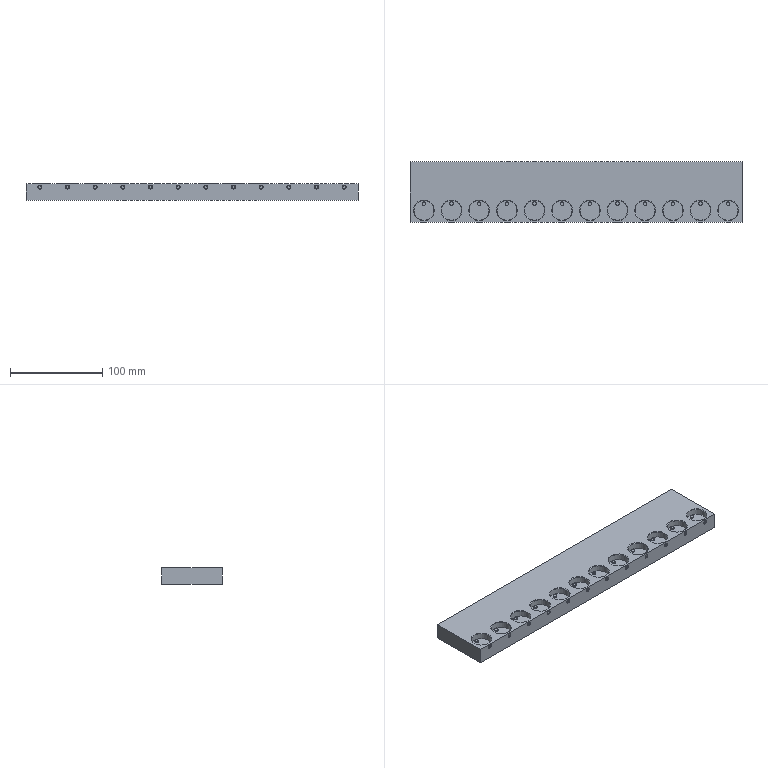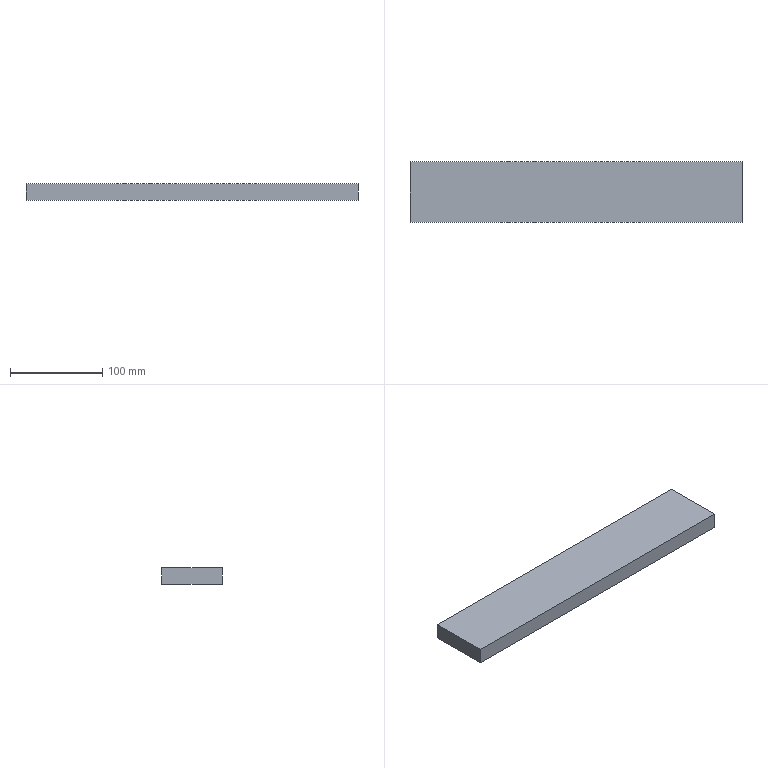CAM job | NX | 3+2 milling, drilling | part box 360 x 66 x 17.6 mm | stock box 360 x 66 x 17.6 mm
Tools:
number,name,description,diameter,corner_radius,flute_length,length,flutes
1,D4-T1,Milling Tool-5 Parameters,4.0,0.0,50.0,75.0,2
2,D1-T2,Milling Tool-5 Parameters,1.0,0.0,50.0,75.0,2
3,D1-T3,Milling Tool-5 Parameters,1.0,0.0,50.0,75.0,2
4,点钻D8-T4,Drilling Tool,8.0,0.0,35.0,50.0,2
5,钻头3.3-T5,Drilling Tool,3.3,0.0,35.0,50.0,2
6,M4-T6,Drilling Tool,3.3,0.0,35.0,50.0,2
Operations:
program,operation,operation_type,tool,method,geometry_group,spindle_rpm,surface_speed,feed_per_tooth,feed_cut,feed_plunge,cut_length_mm,path_length_mm,cut_time_min,machine_time_min
210619,1,CavityMilling,D4-T1,METHOD,WORKPIECE,8000.0,150.0,0.125,2000.0,100.0,3640.257,4036.618,1.82,1.875
210619,1_COPY,CavityMilling,D4-T1,METHOD,WORKPIECE,8000.0,150.0,0.125,2000.0,100.0,3640.257,4036.618,1.82,1.875
210619,1_COPY_1,CavityMilling,D4-T1,METHOD,WORKPIECE,8000.0,150.0,0.125,2000.0,100.0,3640.257,4036.618,1.82,1.875
210619,1_COPY_2,CavityMilling,D4-T1,METHOD,WORKPIECE,8000.0,150.0,0.125,2000.0,100.0,3640.257,4036.618,1.82,1.875
210619,1_COPY_3,CavityMilling,D4-T1,METHOD,WORKPIECE,8000.0,150.0,0.125,2000.0,100.0,3640.257,4036.618,1.82,1.875
210619,1_COPY_4,CavityMilling,D4-T1,METHOD,WORKPIECE,8000.0,150.0,0.125,2000.0,100.0,3640.257,4036.618,1.82,1.875
210619,1_COPY_5,CavityMilling,D4-T1,METHOD,WORKPIECE,8000.0,150.0,0.125,2000.0,100.0,3640.257,4036.618,1.82,1.875
210619,1_COPY_6,CavityMilling,D4-T1,METHOD,WORKPIECE,8000.0,150.0,0.125,2000.0,100.0,3640.257,4036.618,1.82,1.875
210619,1_COPY_7,CavityMilling,D4-T1,METHOD,WORKPIECE,8000.0,150.0,0.125,2000.0,100.0,3640.257,4036.618,1.82,1.875
210619,1_COPY_8,CavityMilling,D4-T1,METHOD,WORKPIECE,8000.0,150.0,0.125,2000.0,100.0,3640.257,4036.618,1.82,1.875
210619,1_COPY_9,CavityMilling,D4-T1,METHOD,WORKPIECE,8000.0,150.0,0.125,2000.0,100.0,3640.257,4036.618,1.82,1.875
210619,1_COPY_10,CavityMilling,D4-T1,METHOD,WORKPIECE,8000.0,150.0,0.125,2000.0,100.0,3640.257,4036.618,1.82,1.875
210619,2,CavityMilling,D1-T2,METHOD,WORKPIECE,8000.0,150.0,0.125,2000.0,100.0,4141.424,4646.25,2.071,2.144
210619,2_COPY,CavityMilling,D1-T2,METHOD,WORKPIECE,8000.0,150.0,0.125,2000.0,100.0,4141.424,4646.25,2.071,2.144
210619,2_COPY_1,CavityMilling,D1-T2,METHOD,WORKPIECE,8000.0,150.0,0.125,2000.0,100.0,4141.424,4646.25,2.071,2.144
210619,2_COPY_2,CavityMilling,D1-T2,METHOD,WORKPIECE,8000.0,150.0,0.125,2000.0,100.0,4141.424,4646.25,2.071,2.144
210619,2_COPY_3,CavityMilling,D1-T2,METHOD,WORKPIECE,8000.0,150.0,0.125,2000.0,100.0,4141.424,4646.25,2.071,2.144
210619,2_COPY_4,CavityMilling,D1-T2,METHOD,WORKPIECE,8000.0,150.0,0.125,2000.0,100.0,4141.424,4646.25,2.071,2.144
210619,2_COPY_5,CavityMilling,D1-T2,METHOD,WORKPIECE,8000.0,150.0,0.125,2000.0,100.0,4141.424,4646.25,2.071,2.144
210619,2_COPY_6,CavityMilling,D1-T2,METHOD,WORKPIECE,8000.0,150.0,0.125,2000.0,100.0,4141.424,4646.25,2.071,2.144
210619,2_COPY_7,CavityMilling,D1-T2,METHOD,WORKPIECE,8000.0,150.0,0.125,2000.0,100.0,4141.424,4646.25,2.071,2.144
210619,2_COPY_8,CavityMilling,D1-T2,METHOD,WORKPIECE,8000.0,150.0,0.125,2000.0,100.0,4141.424,4646.25,2.071,2.144
210619,2_COPY_9,CavityMilling,D1-T2,METHOD,WORKPIECE,8000.0,150.0,0.125,2000.0,100.0,4141.424,4646.25,2.071,2.144
210619,2_COPY_10,CavityMilling,D1-T2,METHOD,WORKPIECE,8000.0,150.0,0.125,2000.0,100.0,4141.424,4646.25,2.071,2.144
210619,3,ZLevelMilling,D1-T3,METHOD,WORKPIECE,6500.0,20.0,0.1923,2500.0,100.0,2438.408,2863.141,0.9754,1.018
210619,3_COPY,ZLevelMilling,D1-T3,METHOD,WORKPIECE,6500.0,20.0,0.1923,2500.0,100.0,2438.408,2863.141,0.9754,1.018
210619,3_COPY_1,ZLevelMilling,D1-T3,METHOD,WORKPIECE,6500.0,20.0,0.1923,2500.0,100.0,2438.408,2863.141,0.9754,1.018
210619,3_COPY_2,ZLevelMilling,D1-T3,METHOD,WORKPIECE,6500.0,20.0,0.1923,2500.0,100.0,2438.408,2863.141,0.9754,1.018
210619,3_COPY_3,ZLevelMilling,D1-T3,METHOD,WORKPIECE,6500.0,20.0,0.1923,2500.0,100.0,2438.408,2863.141,0.9754,1.018
210619,3_COPY_4,ZLevelMilling,D1-T3,METHOD,WORKPIECE,6500.0,20.0,0.1923,2500.0,100.0,2438.408,2863.141,0.9754,1.018
210619,3_COPY_5,ZLevelMilling,D1-T3,METHOD,WORKPIECE,6500.0,20.0,0.1923,2500.0,100.0,2438.408,2863.141,0.9754,1.018
210619,3_COPY_6,ZLevelMilling,D1-T3,METHOD,WORKPIECE,6500.0,20.0,0.1923,2500.0,100.0,2438.408,2863.141,0.9754,1.018
210619,3_COPY_7,ZLevelMilling,D1-T3,METHOD,WORKPIECE,6500.0,20.0,0.1923,2500.0,100.0,2438.408,2863.141,0.9754,1.018
210619,3_COPY_8,ZLevelMilling,D1-T3,METHOD,WORKPIECE,6500.0,20.0,0.1923,2500.0,100.0,2438.408,2863.141,0.9754,1.018
210619,3_COPY_9,ZLevelMilling,D1-T3,METHOD,WORKPIECE,6500.0,20.0,0.1923,2500.0,100.0,2438.408,2863.141,0.9754,1.018
210619,3_COPY_10,ZLevelMilling,D1-T3,METHOD,WORKPIECE,6500.0,20.0,0.1923,2500.0,100.0,2438.408,2863.141,0.9754,1.018
210619,4,VolumeBased25DMillingOperation,D1-T3,METHOD,WORKPIECE,6500.0,0.0,0.0,1000.0,100.0,3123.434,3568.314,7.936,8.002
210619,4_COPY,VolumeBased25DMillingOperation,D1-T3,METHOD,WORKPIECE,6500.0,0.0,0.0,1000.0,100.0,3123.434,3568.314,7.936,8.002
210619,4_COPY_1,VolumeBased25DMillingOperation,D1-T3,METHOD,WORKPIECE,6500.0,0.0,0.0,1000.0,100.0,3123.434,3568.314,7.936,8.002
210619,4_COPY_2,VolumeBased25DMillingOperation,D1-T3,METHOD,WORKPIECE,6500.0,0.0,0.0,1000.0,100.0,3123.434,3568.314,7.936,8.002
210619,4_COPY_3,VolumeBased25DMillingOperation,D1-T3,METHOD,WORKPIECE,6500.0,0.0,0.0,1000.0,100.0,3123.434,3568.314,7.936,8.002
210619,4_COPY_4,VolumeBased25DMillingOperation,D1-T3,METHOD,WORKPIECE,6500.0,0.0,0.0,1000.0,100.0,3123.434,3568.314,7.936,8.002
210619,4_COPY_5,VolumeBased25DMillingOperation,D1-T3,METHOD,WORKPIECE,6500.0,0.0,0.0,1000.0,100.0,3123.434,3568.314,7.936,8.002
210619,4_COPY_6,VolumeBased25DMillingOperation,D1-T3,METHOD,WORKPIECE,6500.0,0.0,0.0,1000.0,100.0,3123.434,3568.314,7.936,8.002
210619,4_COPY_7,VolumeBased25DMillingOperation,D1-T3,METHOD,WORKPIECE,6500.0,0.0,0.0,1000.0,100.0,3123.434,3568.314,7.936,8.002
210619,4_COPY_8,VolumeBased25DMillingOperation,D1-T3,METHOD,WORKPIECE,6500.0,0.0,0.0,1000.0,100.0,3123.434,3568.314,7.936,8.002
210619,4_COPY_9,VolumeBased25DMillingOperation,D1-T3,METHOD,WORKPIECE,6500.0,0.0,0.0,1000.0,100.0,3123.434,3568.314,7.936,8.002
210619,4_COPY_10,VolumeBased25DMillingOperation,D1-T3,METHOD,WORKPIECE,6500.0,0.0,0.0,1000.0,100.0,3123.434,3568.314,7.936,8.002
T1,D1,Operation,点钻D8-T4,METHOD,WORKPIECE_1,5000.0,125.0,0.025,250.0,0.0,38.4,444.446,0.1536,0.1942
T1,D2,Operation,钻头3.3-T5,METHOD,WORKPIECE_1,1500.0,15.0,0.05,150.0,0.0,108.0,583.646,0.72,0.7676
T1,D3,Operation,M4-T6,METHOD,WORKPIECE_1,300.0,3.0,0.0012,0.7,0.0,108.0,583.646,154.286,154.333